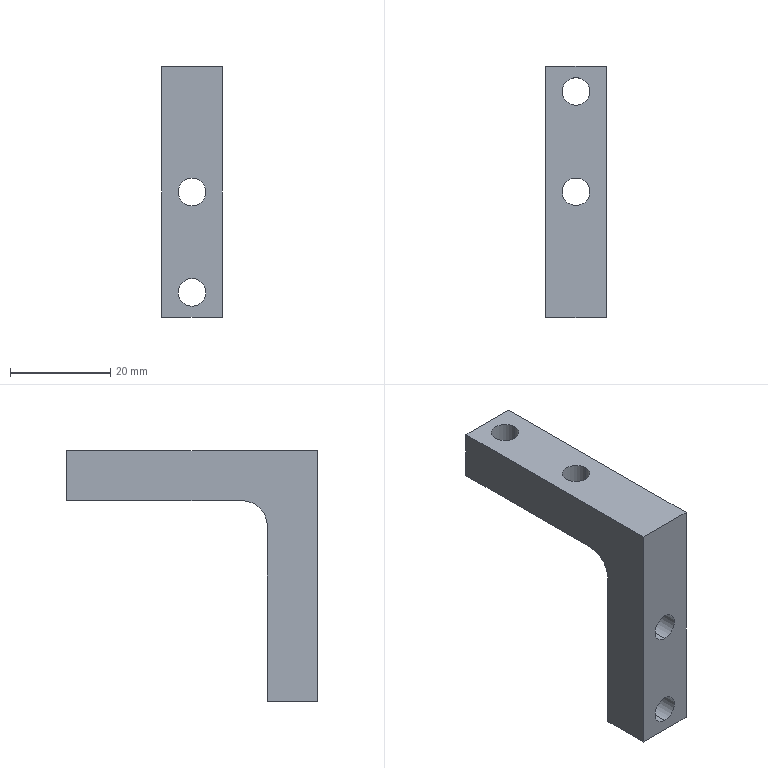Part | SolidWorks | features HoleWzd 2, Extrusion 1, Fillet 1 | 1 solid | 17 faces | box 12 x 50 x 50 mm | volume 9914 mm3 | cylinder 9 | plane 8 | commonest cylinder face diameters 5.5 x8 10 x1
STEP:
#1=CARTESIAN_POINT('',(6.,0.,-27.75));
#2=VERTEX_POINT('',#1);
#3=CARTESIAN_POINT('',(6.,0.,-22.25));
#4=VERTEX_POINT('',#3);
#5=CARTESIAN_POINT('',(6.,0.,-25.));
#6=DIRECTION('',(0.,1.,0.));
#7=DIRECTION('',(0.,0.,1.));
#8=AXIS2_PLACEMENT_3D('',#5,#6,#7);
#9=CIRCLE('',#8,2.75);
#10=EDGE_CURVE('',#2,#4,#9,.T.);
#11=ORIENTED_EDGE('',*,*,#10,.F.);
#12=CARTESIAN_POINT('',(6.,10.,-27.75));
#13=VERTEX_POINT('',#12);
#14=CARTESIAN_POINT('',(6.,10.,-27.75));
#15=DIRECTION('',(0.,1.,0.));
#16=VECTOR('',#15,1000.);
#17=LINE('',#14,#16);
#18=EDGE_CURVE('',#2,#13,#17,.T.);
#19=ORIENTED_EDGE('',*,*,#18,.T.);
#20=CARTESIAN_POINT('',(6.,10.,-22.25));
#21=VERTEX_POINT('',#20);
#22=CARTESIAN_POINT('',(6.,10.,-25.));
#23=DIRECTION('',(0.,1.,0.));
#24=DIRECTION('',(0.,0.,1.));
#25=AXIS2_PLACEMENT_3D('',#22,#23,#24);
#26=CIRCLE('',#25,2.75);
#27=EDGE_CURVE('',#13,#21,#26,.T.);
#28=ORIENTED_EDGE('',*,*,#27,.T.);
#29=CARTESIAN_POINT('',(6.,10.,-22.25));
#30=DIRECTION('',(0.,1.,0.));
#31=VECTOR('',#30,1000.);
#32=LINE('',#29,#31);
#33=EDGE_CURVE('',#4,#21,#32,.T.);
#34=ORIENTED_EDGE('',*,*,#33,.F.);
#35=EDGE_LOOP('',(#11,#19,#28,#34));
#36=FACE_OUTER_BOUND('',#35,.T.);
#37=CARTESIAN_POINT('',(6.,10.,-25.));
#38=DIRECTION('',(0.,1.,0.));
#39=DIRECTION('',(0.,0.,1.));
#40=AXIS2_PLACEMENT_3D('',#37,#38,#39);
#41=CYLINDRICAL_SURFACE('',#40,2.75);
#42=ADVANCED_FACE('',(#36),#41,.F.);
#43=CARTESIAN_POINT('',(6.,0.,-47.75));
#44=VERTEX_POINT('',#43);
#45=CARTESIAN_POINT('',(6.,0.,-42.25));
#46=VERTEX_POINT('',#45);
#47=CARTESIAN_POINT('',(6.,0.,-45.));
#48=DIRECTION('',(0.,1.,0.));
#49=DIRECTION('',(0.,0.,1.));
#50=AXIS2_PLACEMENT_3D('',#47,#48,#49);
#51=CIRCLE('',#50,2.75);
#52=EDGE_CURVE('',#44,#46,#51,.T.);
#53=ORIENTED_EDGE('',*,*,#52,.F.);
#54=CARTESIAN_POINT('',(6.,10.,-47.75));
#55=VERTEX_POINT('',#54);
#56=CARTESIAN_POINT('',(6.,10.,-47.75));
#57=DIRECTION('',(0.,1.,0.));
#58=VECTOR('',#57,1000.);
#59=LINE('',#56,#58);
#60=EDGE_CURVE('',#44,#55,#59,.T.);
#61=ORIENTED_EDGE('',*,*,#60,.T.);
#62=CARTESIAN_POINT('',(6.,10.,-42.25));
#63=VERTEX_POINT('',#62);
#64=CARTESIAN_POINT('',(6.,10.,-45.));
#65=DIRECTION('',(0.,1.,0.));
#66=DIRECTION('',(0.,0.,1.));
#67=AXIS2_PLACEMENT_3D('',#64,#65,#66);
#68=CIRCLE('',#67,2.75);
#69=EDGE_CURVE('',#55,#63,#68,.T.);
#70=ORIENTED_EDGE('',*,*,#69,.T.);
#71=CARTESIAN_POINT('',(6.,10.,-42.25));
#72=DIRECTION('',(0.,1.,0.));
#73=VECTOR('',#72,1000.);
#74=LINE('',#71,#73);
#75=EDGE_CURVE('',#46,#63,#74,.T.);
#76=ORIENTED_EDGE('',*,*,#75,.F.);
#77=EDGE_LOOP('',(#53,#61,#70,#76));
#78=FACE_OUTER_BOUND('',#77,.T.);
#79=CARTESIAN_POINT('',(6.,10.,-45.));
#80=DIRECTION('',(0.,1.,0.));
#81=DIRECTION('',(0.,0.,1.));
#82=AXIS2_PLACEMENT_3D('',#79,#80,#81);
#83=CYLINDRICAL_SURFACE('',#82,2.75);
#84=ADVANCED_FACE('',(#78),#83,.F.);
#85=CARTESIAN_POINT('',(8.75,45.,0.));
#86=VERTEX_POINT('',#85);
#87=CARTESIAN_POINT('',(3.25,45.,0.));
#88=VERTEX_POINT('',#87);
#89=CARTESIAN_POINT('',(6.,45.,0.));
#90=DIRECTION('',(0.,0.,-1.));
#91=DIRECTION('',(-1.,0.,0.));
#92=AXIS2_PLACEMENT_3D('',#89,#90,#91);
#93=CIRCLE('',#92,2.75);
#94=EDGE_CURVE('',#86,#88,#93,.T.);
#95=ORIENTED_EDGE('',*,*,#94,.F.);
#96=CARTESIAN_POINT('',(8.75,45.,-10.));
#97=VERTEX_POINT('',#96);
#98=CARTESIAN_POINT('',(8.75,45.,-10.));
#99=DIRECTION('',(0.,0.,-1.));
#100=VECTOR('',#99,1000.);
#101=LINE('',#98,#100);
#102=EDGE_CURVE('',#86,#97,#101,.T.);
#103=ORIENTED_EDGE('',*,*,#102,.T.);
#104=CARTESIAN_POINT('',(3.25,45.,-10.));
#105=VERTEX_POINT('',#104);
#106=CARTESIAN_POINT('',(6.,45.,-10.));
#107=DIRECTION('',(0.,0.,-1.));
#108=DIRECTION('',(-1.,0.,0.));
#109=AXIS2_PLACEMENT_3D('',#106,#107,#108);
#110=CIRCLE('',#109,2.75);
#111=EDGE_CURVE('',#97,#105,#110,.T.);
#112=ORIENTED_EDGE('',*,*,#111,.T.);
#113=CARTESIAN_POINT('',(3.25,45.,-10.));
#114=DIRECTION('',(0.,0.,-1.));
#115=VECTOR('',#114,1000.);
#116=LINE('',#113,#115);
#117=EDGE_CURVE('',#88,#105,#116,.T.);
#118=ORIENTED_EDGE('',*,*,#117,.F.);
#119=EDGE_LOOP('',(#95,#103,#112,#118));
#120=FACE_OUTER_BOUND('',#119,.T.);
#121=CARTESIAN_POINT('',(6.,45.,-10.));
#122=DIRECTION('',(0.,0.,-1.));
#123=DIRECTION('',(-1.,0.,0.));
#124=AXIS2_PLACEMENT_3D('',#121,#122,#123);
#125=CYLINDRICAL_SURFACE('',#124,2.75);
#126=ADVANCED_FACE('',(#120),#125,.F.);
#127=CARTESIAN_POINT('',(8.75,25.,0.));
#128=VERTEX_POINT('',#127);
#129=CARTESIAN_POINT('',(3.25,25.,0.));
#130=VERTEX_POINT('',#129);
#131=CARTESIAN_POINT('',(6.,25.,0.));
#132=DIRECTION('',(0.,0.,-1.));
#133=DIRECTION('',(-1.,0.,0.));
#134=AXIS2_PLACEMENT_3D('',#131,#132,#133);
#135=CIRCLE('',#134,2.75);
#136=EDGE_CURVE('',#128,#130,#135,.T.);
#137=ORIENTED_EDGE('',*,*,#136,.F.);
#138=CARTESIAN_POINT('',(8.75,25.,-10.));
#139=VERTEX_POINT('',#138);
#140=CARTESIAN_POINT('',(8.75,25.,-10.));
#141=DIRECTION('',(0.,0.,-1.));
#142=VECTOR('',#141,1000.);
#143=LINE('',#140,#142);
#144=EDGE_CURVE('',#128,#139,#143,.T.);
#145=ORIENTED_EDGE('',*,*,#144,.T.);
#146=CARTESIAN_POINT('',(3.25,25.,-10.));
#147=VERTEX_POINT('',#146);
#148=CARTESIAN_POINT('',(6.,25.,-10.));
#149=DIRECTION('',(0.,0.,-1.));
#150=DIRECTION('',(-1.,0.,0.));
#151=AXIS2_PLACEMENT_3D('',#148,#149,#150);
#152=CIRCLE('',#151,2.75);
#153=EDGE_CURVE('',#139,#147,#152,.T.);
#154=ORIENTED_EDGE('',*,*,#153,.T.);
#155=CARTESIAN_POINT('',(3.25,25.,-10.));
#156=DIRECTION('',(0.,0.,-1.));
#157=VECTOR('',#156,1000.);
#158=LINE('',#155,#157);
#159=EDGE_CURVE('',#130,#147,#158,.T.);
#160=ORIENTED_EDGE('',*,*,#159,.F.);
#161=EDGE_LOOP('',(#137,#145,#154,#160));
#162=FACE_OUTER_BOUND('',#161,.T.);
#163=CARTESIAN_POINT('',(6.,25.,-10.));
#164=DIRECTION('',(0.,0.,-1.));
#165=DIRECTION('',(-1.,0.,0.));
#166=AXIS2_PLACEMENT_3D('',#163,#164,#165);
#167=CYLINDRICAL_SURFACE('',#166,2.75);
#168=ADVANCED_FACE('',(#162),#167,.F.);
#169=CARTESIAN_POINT('',(6.,0.,-25.));
#170=DIRECTION('',(0.,1.,0.));
#171=DIRECTION('',(0.,0.,1.));
#172=AXIS2_PLACEMENT_3D('',#169,#170,#171);
#173=CIRCLE('',#172,2.75);
#174=EDGE_CURVE('',#4,#2,#173,.T.);
#175=ORIENTED_EDGE('',*,*,#174,.T.);
#176=ORIENTED_EDGE('',*,*,#10,.T.);
#177=EDGE_LOOP('',(#175,#176));
#178=FACE_BOUND('',#177,.T.);
#179=CARTESIAN_POINT('',(6.,0.,-45.));
#180=DIRECTION('',(0.,1.,0.));
#181=DIRECTION('',(0.,0.,1.));
#182=AXIS2_PLACEMENT_3D('',#179,#180,#181);
#183=CIRCLE('',#182,2.75);
#184=EDGE_CURVE('',#46,#44,#183,.T.);
#185=ORIENTED_EDGE('',*,*,#184,.T.);
#186=ORIENTED_EDGE('',*,*,#52,.T.);
#187=EDGE_LOOP('',(#185,#186));
#188=FACE_BOUND('',#187,.T.);
#189=CARTESIAN_POINT('',(0.,0.,0.));
#190=VERTEX_POINT('',#189);
#191=CARTESIAN_POINT('',(0.,0.,-50.));
#192=VERTEX_POINT('',#191);
#193=CARTESIAN_POINT('',(0.,0.,-50.));
#194=DIRECTION('',(0.,0.,-1.));
#195=VECTOR('',#194,1000.);
#196=LINE('',#193,#195);
#197=EDGE_CURVE('',#190,#192,#196,.T.);
#198=ORIENTED_EDGE('',*,*,#197,.T.);
#199=CARTESIAN_POINT('',(12.,0.,-50.));
#200=VERTEX_POINT('',#199);
#201=CARTESIAN_POINT('',(12.,0.,-50.));
#202=DIRECTION('',(-1.,0.,0.));
#203=VECTOR('',#202,1000.);
#204=LINE('',#201,#203);
#205=EDGE_CURVE('',#200,#192,#204,.T.);
#206=ORIENTED_EDGE('',*,*,#205,.F.);
#207=CARTESIAN_POINT('',(12.,0.,0.));
#208=VERTEX_POINT('',#207);
#209=CARTESIAN_POINT('',(12.,0.,-50.));
#210=DIRECTION('',(0.,0.,-1.));
#211=VECTOR('',#210,1000.);
#212=LINE('',#209,#211);
#213=EDGE_CURVE('',#208,#200,#212,.T.);
#214=ORIENTED_EDGE('',*,*,#213,.F.);
#215=CARTESIAN_POINT('',(12.,0.,0.));
#216=DIRECTION('',(-1.,0.,0.));
#217=VECTOR('',#216,1000.);
#218=LINE('',#215,#217);
#219=EDGE_CURVE('',#208,#190,#218,.T.);
#220=ORIENTED_EDGE('',*,*,#219,.T.);
#221=EDGE_LOOP('',(#198,#206,#214,#220));
#222=FACE_OUTER_BOUND('',#221,.T.);
#223=CARTESIAN_POINT('',(12.,0.,-50.));
#224=DIRECTION('',(0.,1.,0.));
#225=DIRECTION('',(0.,0.,1.));
#226=AXIS2_PLACEMENT_3D('',#223,#224,#225);
#227=PLANE('',#226);
#228=ADVANCED_FACE('',(#178,#188,#222),#227,.F.);
#229=CARTESIAN_POINT('',(0.,10.,-50.));
#230=VERTEX_POINT('',#229);
#231=CARTESIAN_POINT('',(0.,10.,-50.));
#232=DIRECTION('',(0.,1.,0.));
#233=VECTOR('',#232,1000.);
#234=LINE('',#231,#233);
#235=EDGE_CURVE('',#192,#230,#234,.T.);
#236=ORIENTED_EDGE('',*,*,#235,.T.);
#237=CARTESIAN_POINT('',(12.,10.,-50.));
#238=VERTEX_POINT('',#237);
#239=CARTESIAN_POINT('',(12.,10.,-50.));
#240=DIRECTION('',(-1.,0.,0.));
#241=VECTOR('',#240,1000.);
#242=LINE('',#239,#241);
#243=EDGE_CURVE('',#238,#230,#242,.T.);
#244=ORIENTED_EDGE('',*,*,#243,.F.);
#245=CARTESIAN_POINT('',(12.,10.,-50.));
#246=DIRECTION('',(0.,1.,0.));
#247=VECTOR('',#246,1000.);
#248=LINE('',#245,#247);
#249=EDGE_CURVE('',#200,#238,#248,.T.);
#250=ORIENTED_EDGE('',*,*,#249,.F.);
#251=ORIENTED_EDGE('',*,*,#205,.T.);
#252=EDGE_LOOP('',(#236,#244,#250,#251));
#253=FACE_OUTER_BOUND('',#252,.T.);
#254=CARTESIAN_POINT('',(12.,10.,-50.));
#255=DIRECTION('',(0.,0.,1.));
#256=DIRECTION('',(1.,0.,0.));
#257=AXIS2_PLACEMENT_3D('',#254,#255,#256);
#258=PLANE('',#257);
#259=ADVANCED_FACE('',(#253),#258,.F.);
#260=CARTESIAN_POINT('',(6.,10.,-25.));
#261=DIRECTION('',(0.,1.,0.));
#262=DIRECTION('',(0.,0.,1.));
#263=AXIS2_PLACEMENT_3D('',#260,#261,#262);
#264=CIRCLE('',#263,2.75);
#265=EDGE_CURVE('',#21,#13,#264,.T.);
#266=ORIENTED_EDGE('',*,*,#265,.F.);
#267=ORIENTED_EDGE('',*,*,#27,.F.);
#268=EDGE_LOOP('',(#266,#267));
#269=FACE_BOUND('',#268,.T.);
#270=CARTESIAN_POINT('',(6.,10.,-45.));
#271=DIRECTION('',(0.,1.,0.));
#272=DIRECTION('',(0.,0.,1.));
#273=AXIS2_PLACEMENT_3D('',#270,#271,#272);
#274=CIRCLE('',#273,2.75);
#275=EDGE_CURVE('',#63,#55,#274,.T.);
#276=ORIENTED_EDGE('',*,*,#275,.F.);
#277=ORIENTED_EDGE('',*,*,#69,.F.);
#278=EDGE_LOOP('',(#276,#277));
#279=FACE_BOUND('',#278,.T.);
#280=CARTESIAN_POINT('',(0.,10.,-15.));
#281=VERTEX_POINT('',#280);
#282=CARTESIAN_POINT('',(0.,10.,-10.));
#283=DIRECTION('',(0.,0.,1.));
#284=VECTOR('',#283,1000.);
#285=LINE('',#282,#284);
#286=EDGE_CURVE('',#230,#281,#285,.T.);
#287=ORIENTED_EDGE('',*,*,#286,.T.);
#288=CARTESIAN_POINT('',(12.,10.,-15.));
#289=VERTEX_POINT('',#288);
#290=CARTESIAN_POINT('',(12.,10.,-15.));
#291=DIRECTION('',(1.,0.,0.));
#292=VECTOR('',#291,1000.);
#293=LINE('',#290,#292);
#294=EDGE_CURVE('',#281,#289,#293,.T.);
#295=ORIENTED_EDGE('',*,*,#294,.T.);
#296=CARTESIAN_POINT('',(12.,10.,-10.));
#297=DIRECTION('',(0.,0.,1.));
#298=VECTOR('',#297,1000.);
#299=LINE('',#296,#298);
#300=EDGE_CURVE('',#238,#289,#299,.T.);
#301=ORIENTED_EDGE('',*,*,#300,.F.);
#302=ORIENTED_EDGE('',*,*,#243,.T.);
#303=EDGE_LOOP('',(#287,#295,#301,#302));
#304=FACE_OUTER_BOUND('',#303,.T.);
#305=CARTESIAN_POINT('',(12.,10.,-10.));
#306=DIRECTION('',(0.,-1.,0.));
#307=DIRECTION('',(0.,0.,-1.));
#308=AXIS2_PLACEMENT_3D('',#305,#306,#307);
#309=PLANE('',#308);
#310=ADVANCED_FACE('',(#269,#279,#304),#309,.F.);
#311=CARTESIAN_POINT('',(6.,45.,-10.));
#312=DIRECTION('',(0.,0.,-1.));
#313=DIRECTION('',(-1.,0.,0.));
#314=AXIS2_PLACEMENT_3D('',#311,#312,#313);
#315=CIRCLE('',#314,2.75);
#316=EDGE_CURVE('',#105,#97,#315,.T.);
#317=ORIENTED_EDGE('',*,*,#316,.F.);
#318=ORIENTED_EDGE('',*,*,#111,.F.);
#319=EDGE_LOOP('',(#317,#318));
#320=FACE_BOUND('',#319,.T.);
#321=CARTESIAN_POINT('',(6.,25.,-10.));
#322=DIRECTION('',(0.,0.,-1.));
#323=DIRECTION('',(-1.,0.,0.));
#324=AXIS2_PLACEMENT_3D('',#321,#322,#323);
#325=CIRCLE('',#324,2.75);
#326=EDGE_CURVE('',#147,#139,#325,.T.);
#327=ORIENTED_EDGE('',*,*,#326,.F.);
#328=ORIENTED_EDGE('',*,*,#153,.F.);
#329=EDGE_LOOP('',(#327,#328));
#330=FACE_BOUND('',#329,.T.);
#331=CARTESIAN_POINT('',(12.,15.,-10.));
#332=VERTEX_POINT('',#331);
#333=CARTESIAN_POINT('',(12.,50.,-10.));
#334=VERTEX_POINT('',#333);
#335=CARTESIAN_POINT('',(12.,50.,-10.));
#336=DIRECTION('',(0.,1.,0.));
#337=VECTOR('',#336,1000.);
#338=LINE('',#335,#337);
#339=EDGE_CURVE('',#332,#334,#338,.T.);
#340=ORIENTED_EDGE('',*,*,#339,.F.);
#341=CARTESIAN_POINT('',(0.,15.,-10.));
#342=VERTEX_POINT('',#341);
#343=CARTESIAN_POINT('',(0.,15.,-10.));
#344=DIRECTION('',(-1.,0.,0.));
#345=VECTOR('',#344,1000.);
#346=LINE('',#343,#345);
#347=EDGE_CURVE('',#332,#342,#346,.T.);
#348=ORIENTED_EDGE('',*,*,#347,.T.);
#349=CARTESIAN_POINT('',(0.,50.,-10.));
#350=VERTEX_POINT('',#349);
#351=CARTESIAN_POINT('',(0.,50.,-10.));
#352=DIRECTION('',(0.,1.,0.));
#353=VECTOR('',#352,1000.);
#354=LINE('',#351,#353);
#355=EDGE_CURVE('',#342,#350,#354,.T.);
#356=ORIENTED_EDGE('',*,*,#355,.T.);
#357=CARTESIAN_POINT('',(12.,50.,-10.));
#358=DIRECTION('',(-1.,0.,0.));
#359=VECTOR('',#358,1000.);
#360=LINE('',#357,#359);
#361=EDGE_CURVE('',#334,#350,#360,.T.);
#362=ORIENTED_EDGE('',*,*,#361,.F.);
#363=EDGE_LOOP('',(#340,#348,#356,#362));
#364=FACE_OUTER_BOUND('',#363,.T.);
#365=CARTESIAN_POINT('',(12.,50.,-10.));
#366=DIRECTION('',(0.,0.,1.));
#367=DIRECTION('',(1.,0.,0.));
#368=AXIS2_PLACEMENT_3D('',#365,#366,#367);
#369=PLANE('',#368);
#370=ADVANCED_FACE('',(#320,#330,#364),#369,.F.);
#371=CARTESIAN_POINT('',(0.,50.,0.));
#372=VERTEX_POINT('',#371);
#373=CARTESIAN_POINT('',(0.,50.,0.));
#374=DIRECTION('',(0.,0.,1.));
#375=VECTOR('',#374,1000.);
#376=LINE('',#373,#375);
#377=EDGE_CURVE('',#350,#372,#376,.T.);
#378=ORIENTED_EDGE('',*,*,#377,.T.);
#379=CARTESIAN_POINT('',(12.,50.,0.));
#380=VERTEX_POINT('',#379);
#381=CARTESIAN_POINT('',(12.,50.,0.));
#382=DIRECTION('',(-1.,0.,0.));
#383=VECTOR('',#382,1000.);
#384=LINE('',#381,#383);
#385=EDGE_CURVE('',#380,#372,#384,.T.);
#386=ORIENTED_EDGE('',*,*,#385,.F.);
#387=CARTESIAN_POINT('',(12.,50.,0.));
#388=DIRECTION('',(0.,0.,1.));
#389=VECTOR('',#388,1000.);
#390=LINE('',#387,#389);
#391=EDGE_CURVE('',#334,#380,#390,.T.);
#392=ORIENTED_EDGE('',*,*,#391,.F.);
#393=ORIENTED_EDGE('',*,*,#361,.T.);
#394=EDGE_LOOP('',(#378,#386,#392,#393));
#395=FACE_OUTER_BOUND('',#394,.T.);
#396=CARTESIAN_POINT('',(12.,50.,0.));
#397=DIRECTION('',(0.,-1.,0.));
#398=DIRECTION('',(0.,0.,-1.));
#399=AXIS2_PLACEMENT_3D('',#396,#397,#398);
#400=PLANE('',#399);
#401=ADVANCED_FACE('',(#395),#400,.F.);
#402=CARTESIAN_POINT('',(6.,45.,0.));
#403=DIRECTION('',(0.,0.,-1.));
#404=DIRECTION('',(-1.,0.,0.));
#405=AXIS2_PLACEMENT_3D('',#402,#403,#404);
#406=CIRCLE('',#405,2.75);
#407=EDGE_CURVE('',#88,#86,#406,.T.);
#408=ORIENTED_EDGE('',*,*,#407,.T.);
#409=ORIENTED_EDGE('',*,*,#94,.T.);
#410=EDGE_LOOP('',(#408,#409));
#411=FACE_BOUND('',#410,.T.);
#412=CARTESIAN_POINT('',(6.,25.,0.));
#413=DIRECTION('',(0.,0.,-1.));
#414=DIRECTION('',(-1.,0.,0.));
#415=AXIS2_PLACEMENT_3D('',#412,#413,#414);
#416=CIRCLE('',#415,2.75);
#417=EDGE_CURVE('',#130,#128,#416,.T.);
#418=ORIENTED_EDGE('',*,*,#417,.T.);
#419=ORIENTED_EDGE('',*,*,#136,.T.);
#420=EDGE_LOOP('',(#418,#419));
#421=FACE_BOUND('',#420,.T.);
#422=CARTESIAN_POINT('',(0.,0.,0.));
#423=DIRECTION('',(0.,-1.,0.));
#424=VECTOR('',#423,1000.);
#425=LINE('',#422,#424);
#426=EDGE_CURVE('',#372,#190,#425,.T.);
#427=ORIENTED_EDGE('',*,*,#426,.T.);
#428=ORIENTED_EDGE('',*,*,#219,.F.);
#429=CARTESIAN_POINT('',(12.,0.,0.));
#430=DIRECTION('',(0.,-1.,0.));
#431=VECTOR('',#430,1000.);
#432=LINE('',#429,#431);
#433=EDGE_CURVE('',#380,#208,#432,.T.);
#434=ORIENTED_EDGE('',*,*,#433,.F.);
#435=ORIENTED_EDGE('',*,*,#385,.T.);
#436=EDGE_LOOP('',(#427,#428,#434,#435));
#437=FACE_OUTER_BOUND('',#436,.T.);
#438=CARTESIAN_POINT('',(12.,0.,0.));
#439=DIRECTION('',(0.,0.,-1.));
#440=DIRECTION('',(-1.,0.,0.));
#441=AXIS2_PLACEMENT_3D('',#438,#439,#440);
#442=PLANE('',#441);
#443=ADVANCED_FACE('',(#411,#421,#437),#442,.F.);
#444=ORIENTED_EDGE('',*,*,#213,.T.);
#445=ORIENTED_EDGE('',*,*,#249,.T.);
#446=ORIENTED_EDGE('',*,*,#300,.T.);
#447=CARTESIAN_POINT('',(12.,15.,-15.));
#448=DIRECTION('',(-1.,0.,0.));
#449=DIRECTION('',(0.,0.,1.));
#450=AXIS2_PLACEMENT_3D('',#447,#448,#449);
#451=CIRCLE('',#450,5.);
#452=EDGE_CURVE('',#289,#332,#451,.T.);
#453=ORIENTED_EDGE('',*,*,#452,.T.);
#454=ORIENTED_EDGE('',*,*,#339,.T.);
#455=ORIENTED_EDGE('',*,*,#391,.T.);
#456=ORIENTED_EDGE('',*,*,#433,.T.);
#457=EDGE_LOOP('',(#444,#445,#446,#453,#454,#455,#456));
#458=FACE_OUTER_BOUND('',#457,.T.);
#459=CARTESIAN_POINT('',(12.,0.,0.));
#460=DIRECTION('',(-1.,0.,0.));
#461=DIRECTION('',(0.,0.,1.));
#462=AXIS2_PLACEMENT_3D('',#459,#460,#461);
#463=PLANE('',#462);
#464=ADVANCED_FACE('',(#458),#463,.F.);
#465=ORIENTED_EDGE('',*,*,#197,.F.);
#466=ORIENTED_EDGE('',*,*,#426,.F.);
#467=ORIENTED_EDGE('',*,*,#377,.F.);
#468=ORIENTED_EDGE('',*,*,#355,.F.);
#469=CARTESIAN_POINT('',(0.,15.,-15.));
#470=DIRECTION('',(1.,0.,0.));
#471=DIRECTION('',(0.,0.,1.));
#472=AXIS2_PLACEMENT_3D('',#469,#470,#471);
#473=CIRCLE('',#472,5.);
#474=EDGE_CURVE('',#342,#281,#473,.T.);
#475=ORIENTED_EDGE('',*,*,#474,.T.);
#476=ORIENTED_EDGE('',*,*,#286,.F.);
#477=ORIENTED_EDGE('',*,*,#235,.F.);
#478=EDGE_LOOP('',(#465,#466,#467,#468,#475,#476,#477));
#479=FACE_OUTER_BOUND('',#478,.T.);
#480=CARTESIAN_POINT('',(0.,0.,0.));
#481=DIRECTION('',(-1.,0.,0.));
#482=DIRECTION('',(0.,0.,1.));
#483=AXIS2_PLACEMENT_3D('',#480,#481,#482);
#484=PLANE('',#483);
#485=ADVANCED_FACE('',(#479),#484,.T.);
#486=ORIENTED_EDGE('',*,*,#452,.F.);
#487=ORIENTED_EDGE('',*,*,#294,.F.);
#488=ORIENTED_EDGE('',*,*,#474,.F.);
#489=ORIENTED_EDGE('',*,*,#347,.F.);
#490=EDGE_LOOP('',(#486,#487,#488,#489));
#491=FACE_OUTER_BOUND('',#490,.T.);
#492=CARTESIAN_POINT('',(12.,15.,-15.));
#493=DIRECTION('',(1.,0.,0.));
#494=DIRECTION('',(0.,0.,-1.));
#495=AXIS2_PLACEMENT_3D('',#492,#493,#494);
#496=CYLINDRICAL_SURFACE('',#495,5.);
#497=ADVANCED_FACE('',(#491),#496,.F.);
#498=ORIENTED_EDGE('',*,*,#144,.F.);
#499=ORIENTED_EDGE('',*,*,#417,.F.);
#500=ORIENTED_EDGE('',*,*,#159,.T.);
#501=ORIENTED_EDGE('',*,*,#326,.T.);
#502=EDGE_LOOP('',(#498,#499,#500,#501));
#503=FACE_OUTER_BOUND('',#502,.T.);
#504=CARTESIAN_POINT('',(6.,25.,-10.));
#505=DIRECTION('',(0.,0.,-1.));
#506=DIRECTION('',(-1.,0.,0.));
#507=AXIS2_PLACEMENT_3D('',#504,#505,#506);
#508=CYLINDRICAL_SURFACE('',#507,2.75);
#509=ADVANCED_FACE('',(#503),#508,.F.);
#510=ORIENTED_EDGE('',*,*,#102,.F.);
#511=ORIENTED_EDGE('',*,*,#407,.F.);
#512=ORIENTED_EDGE('',*,*,#117,.T.);
#513=ORIENTED_EDGE('',*,*,#316,.T.);
#514=EDGE_LOOP('',(#510,#511,#512,#513));
#515=FACE_OUTER_BOUND('',#514,.T.);
#516=CARTESIAN_POINT('',(6.,45.,-10.));
#517=DIRECTION('',(0.,0.,-1.));
#518=DIRECTION('',(-1.,0.,0.));
#519=AXIS2_PLACEMENT_3D('',#516,#517,#518);
#520=CYLINDRICAL_SURFACE('',#519,2.75);
#521=ADVANCED_FACE('',(#515),#520,.F.);
#522=ORIENTED_EDGE('',*,*,#60,.F.);
#523=ORIENTED_EDGE('',*,*,#184,.F.);
#524=ORIENTED_EDGE('',*,*,#75,.T.);
#525=ORIENTED_EDGE('',*,*,#275,.T.);
#526=EDGE_LOOP('',(#522,#523,#524,#525));
#527=FACE_OUTER_BOUND('',#526,.T.);
#528=CARTESIAN_POINT('',(6.,10.,-45.));
#529=DIRECTION('',(0.,1.,0.));
#530=DIRECTION('',(0.,0.,1.));
#531=AXIS2_PLACEMENT_3D('',#528,#529,#530);
#532=CYLINDRICAL_SURFACE('',#531,2.75);
#533=ADVANCED_FACE('',(#527),#532,.F.);
#534=ORIENTED_EDGE('',*,*,#18,.F.);
#535=ORIENTED_EDGE('',*,*,#174,.F.);
#536=ORIENTED_EDGE('',*,*,#33,.T.);
#537=ORIENTED_EDGE('',*,*,#265,.T.);
#538=EDGE_LOOP('',(#534,#535,#536,#537));
#539=FACE_OUTER_BOUND('',#538,.T.);
#540=CARTESIAN_POINT('',(6.,10.,-25.));
#541=DIRECTION('',(0.,1.,0.));
#542=DIRECTION('',(0.,0.,1.));
#543=AXIS2_PLACEMENT_3D('',#540,#541,#542);
#544=CYLINDRICAL_SURFACE('',#543,2.75);
#545=ADVANCED_FACE('',(#539),#544,.F.);
#546=CLOSED_SHELL('',(#42,#84,#126,#168,#228,#259,#310,#370,#401,#443,#464,#485,#497,#509,#521,#533,#545));
#547=MANIFOLD_SOLID_BREP('',#546);
#548=CARTESIAN_POINT('',(0.,0.,0.));
#549=DIRECTION('',(0.,0.,1.));
#550=DIRECTION('',(1.,0.,0.));
#551=AXIS2_PLACEMENT_3D('',#548,#549,#550);
#552=(LENGTH_UNIT()NAMED_UNIT(*)SI_UNIT(.MILLI.,.METRE.));
#553=UNCERTAINTY_MEASURE_WITH_UNIT(LENGTH_MEASURE(0.00001),#552,'','');
#554=(NAMED_UNIT(*)PLANE_ANGLE_UNIT()SI_UNIT($,.RADIAN.));
#555=(NAMED_UNIT(*)SI_UNIT($,.STERADIAN.)SOLID_ANGLE_UNIT());
#556=(GEOMETRIC_REPRESENTATION_CONTEXT(3)GLOBAL_UNCERTAINTY_ASSIGNED_CONTEXT((#553))GLOBAL_UNIT_ASSIGNED_CONTEXT((#552,#554,#555))REPRESENTATION_CONTEXT('',''));
#557=ADVANCED_BREP_SHAPE_REPRESENTATION('',(#547,#551),#556);